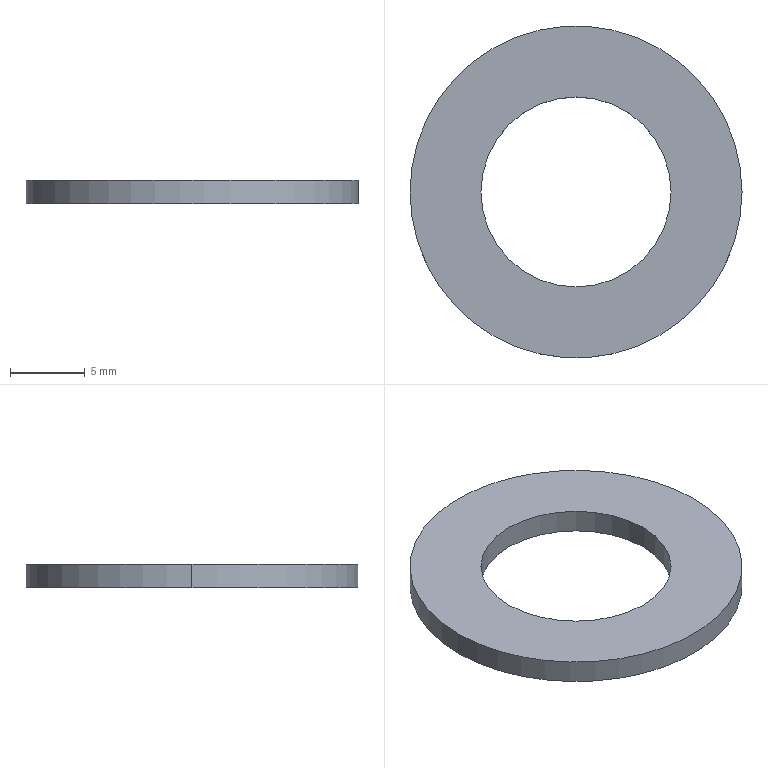Part | SolidWorks | features Extrusion 1 | 1 solid | 6 faces | box 22.276 x 22.276 x 1.6 mm | volume 419.302 mm3 | cylinder 4 | plane 2 | commonest cylinder face diameters 12.751 x2 22.276 x2
STEP:
#1=CARTESIAN_POINT('',(-0.251,0.,0.063));
#2=VERTEX_POINT('',#1);
#3=CARTESIAN_POINT('',(0.251,0.,0.063));
#4=VERTEX_POINT('',#3);
#5=CARTESIAN_POINT('',(0.,0.,0.063));
#6=DIRECTION('',(0.,0.,1.));
#7=DIRECTION('',(1.,0.,0.));
#8=AXIS2_PLACEMENT_3D('',#5,#6,#7);
#9=CIRCLE('',#8,0.251);
#10=EDGE_CURVE('',#2,#4,#9,.T.);
#11=ORIENTED_EDGE('',*,*,#10,.T.);
#12=CARTESIAN_POINT('',(0.251,0.,0.));
#13=VERTEX_POINT('',#12);
#14=CARTESIAN_POINT('',(0.251,0.,0.063));
#15=DIRECTION('',(0.,0.,-1.));
#16=VECTOR('',#15,39.37);
#17=LINE('',#14,#16);
#18=EDGE_CURVE('',#4,#13,#17,.T.);
#19=ORIENTED_EDGE('',*,*,#18,.T.);
#20=CARTESIAN_POINT('',(-0.251,0.,0.));
#21=VERTEX_POINT('',#20);
#22=CARTESIAN_POINT('',(0.,0.,0.));
#23=DIRECTION('',(0.,0.,1.));
#24=DIRECTION('',(1.,0.,0.));
#25=AXIS2_PLACEMENT_3D('',#22,#23,#24);
#26=CIRCLE('',#25,0.251);
#27=EDGE_CURVE('',#21,#13,#26,.T.);
#28=ORIENTED_EDGE('',*,*,#27,.F.);
#29=CARTESIAN_POINT('',(-0.251,0.,0.063));
#30=DIRECTION('',(0.,0.,-1.));
#31=VECTOR('',#30,39.37);
#32=LINE('',#29,#31);
#33=EDGE_CURVE('',#2,#21,#32,.T.);
#34=ORIENTED_EDGE('',*,*,#33,.F.);
#35=EDGE_LOOP('',(#11,#19,#28,#34));
#36=FACE_OUTER_BOUND('',#35,.T.);
#37=CARTESIAN_POINT('',(0.,0.,0.063));
#38=DIRECTION('',(0.,0.,-1.));
#39=DIRECTION('',(-1.,0.,0.));
#40=AXIS2_PLACEMENT_3D('',#37,#38,#39);
#41=CYLINDRICAL_SURFACE('',#40,0.251);
#42=ADVANCED_FACE('',(#36),#41,.F.);
#43=CARTESIAN_POINT('',(0.4385,0.,0.063));
#44=VERTEX_POINT('',#43);
#45=CARTESIAN_POINT('',(-0.4385,0.,0.063));
#46=VERTEX_POINT('',#45);
#47=CARTESIAN_POINT('',(0.,0.,0.063));
#48=DIRECTION('',(0.,0.,1.));
#49=DIRECTION('',(1.,0.,0.));
#50=AXIS2_PLACEMENT_3D('',#47,#48,#49);
#51=CIRCLE('',#50,0.4385);
#52=EDGE_CURVE('',#44,#46,#51,.T.);
#53=ORIENTED_EDGE('',*,*,#52,.F.);
#54=CARTESIAN_POINT('',(0.4385,0.,0.));
#55=VERTEX_POINT('',#54);
#56=CARTESIAN_POINT('',(0.4385,0.,0.063));
#57=DIRECTION('',(0.,0.,-1.));
#58=VECTOR('',#57,39.37);
#59=LINE('',#56,#58);
#60=EDGE_CURVE('',#44,#55,#59,.T.);
#61=ORIENTED_EDGE('',*,*,#60,.T.);
#62=CARTESIAN_POINT('',(-0.4385,0.,0.));
#63=VERTEX_POINT('',#62);
#64=CARTESIAN_POINT('',(0.,0.,0.));
#65=DIRECTION('',(0.,0.,1.));
#66=DIRECTION('',(1.,0.,0.));
#67=AXIS2_PLACEMENT_3D('',#64,#65,#66);
#68=CIRCLE('',#67,0.4385);
#69=EDGE_CURVE('',#55,#63,#68,.T.);
#70=ORIENTED_EDGE('',*,*,#69,.T.);
#71=CARTESIAN_POINT('',(-0.4385,0.,0.063));
#72=DIRECTION('',(0.,0.,-1.));
#73=VECTOR('',#72,39.37);
#74=LINE('',#71,#73);
#75=EDGE_CURVE('',#46,#63,#74,.T.);
#76=ORIENTED_EDGE('',*,*,#75,.F.);
#77=EDGE_LOOP('',(#53,#61,#70,#76));
#78=FACE_OUTER_BOUND('',#77,.T.);
#79=CARTESIAN_POINT('',(0.,0.,0.063));
#80=DIRECTION('',(0.,0.,-1.));
#81=DIRECTION('',(-1.,0.,0.));
#82=AXIS2_PLACEMENT_3D('',#79,#80,#81);
#83=CYLINDRICAL_SURFACE('',#82,0.4385);
#84=ADVANCED_FACE('',(#78),#83,.T.);
#85=CARTESIAN_POINT('',(0.,0.,0.063));
#86=DIRECTION('',(0.,0.,1.));
#87=DIRECTION('',(1.,0.,0.));
#88=AXIS2_PLACEMENT_3D('',#85,#86,#87);
#89=CIRCLE('',#88,0.4385);
#90=EDGE_CURVE('',#46,#44,#89,.T.);
#91=ORIENTED_EDGE('',*,*,#90,.T.);
#92=ORIENTED_EDGE('',*,*,#52,.T.);
#93=EDGE_LOOP('',(#91,#92));
#94=FACE_OUTER_BOUND('',#93,.T.);
#95=ORIENTED_EDGE('',*,*,#10,.F.);
#96=CARTESIAN_POINT('',(0.,0.,0.063));
#97=DIRECTION('',(0.,0.,1.));
#98=DIRECTION('',(1.,0.,0.));
#99=AXIS2_PLACEMENT_3D('',#96,#97,#98);
#100=CIRCLE('',#99,0.251);
#101=EDGE_CURVE('',#4,#2,#100,.T.);
#102=ORIENTED_EDGE('',*,*,#101,.F.);
#103=EDGE_LOOP('',(#95,#102));
#104=FACE_BOUND('',#103,.T.);
#105=CARTESIAN_POINT('',(0.,0.,0.063));
#106=DIRECTION('',(0.,0.,1.));
#107=DIRECTION('',(1.,0.,0.));
#108=AXIS2_PLACEMENT_3D('',#105,#106,#107);
#109=PLANE('',#108);
#110=ADVANCED_FACE('',(#94,#104),#109,.T.);
#111=CARTESIAN_POINT('',(0.,0.,0.));
#112=DIRECTION('',(0.,0.,1.));
#113=DIRECTION('',(1.,0.,0.));
#114=AXIS2_PLACEMENT_3D('',#111,#112,#113);
#115=CIRCLE('',#114,0.4385);
#116=EDGE_CURVE('',#63,#55,#115,.T.);
#117=ORIENTED_EDGE('',*,*,#116,.F.);
#118=ORIENTED_EDGE('',*,*,#69,.F.);
#119=EDGE_LOOP('',(#117,#118));
#120=FACE_OUTER_BOUND('',#119,.T.);
#121=ORIENTED_EDGE('',*,*,#27,.T.);
#122=CARTESIAN_POINT('',(0.,0.,0.));
#123=DIRECTION('',(0.,0.,1.));
#124=DIRECTION('',(1.,0.,0.));
#125=AXIS2_PLACEMENT_3D('',#122,#123,#124);
#126=CIRCLE('',#125,0.251);
#127=EDGE_CURVE('',#13,#21,#126,.T.);
#128=ORIENTED_EDGE('',*,*,#127,.T.);
#129=EDGE_LOOP('',(#121,#128));
#130=FACE_BOUND('',#129,.T.);
#131=CARTESIAN_POINT('',(0.,0.,0.));
#132=DIRECTION('',(0.,0.,1.));
#133=DIRECTION('',(1.,0.,0.));
#134=AXIS2_PLACEMENT_3D('',#131,#132,#133);
#135=PLANE('',#134);
#136=ADVANCED_FACE('',(#120,#130),#135,.F.);
#137=ORIENTED_EDGE('',*,*,#60,.F.);
#138=ORIENTED_EDGE('',*,*,#90,.F.);
#139=ORIENTED_EDGE('',*,*,#75,.T.);
#140=ORIENTED_EDGE('',*,*,#116,.T.);
#141=EDGE_LOOP('',(#137,#138,#139,#140));
#142=FACE_OUTER_BOUND('',#141,.T.);
#143=CARTESIAN_POINT('',(0.,0.,0.063));
#144=DIRECTION('',(0.,0.,-1.));
#145=DIRECTION('',(-1.,0.,0.));
#146=AXIS2_PLACEMENT_3D('',#143,#144,#145);
#147=CYLINDRICAL_SURFACE('',#146,0.4385);
#148=ADVANCED_FACE('',(#142),#147,.T.);
#149=ORIENTED_EDGE('',*,*,#18,.F.);
#150=ORIENTED_EDGE('',*,*,#101,.T.);
#151=ORIENTED_EDGE('',*,*,#33,.T.);
#152=ORIENTED_EDGE('',*,*,#127,.F.);
#153=EDGE_LOOP('',(#149,#150,#151,#152));
#154=FACE_OUTER_BOUND('',#153,.T.);
#155=CARTESIAN_POINT('',(0.,0.,0.063));
#156=DIRECTION('',(0.,0.,-1.));
#157=DIRECTION('',(-1.,0.,0.));
#158=AXIS2_PLACEMENT_3D('',#155,#156,#157);
#159=CYLINDRICAL_SURFACE('',#158,0.251);
#160=ADVANCED_FACE('',(#154),#159,.F.);
#161=CLOSED_SHELL('',(#42,#84,#110,#136,#148,#160));
#162=MANIFOLD_SOLID_BREP('',#161);
#163=CARTESIAN_POINT('',(0.,0.,0.));
#164=DIRECTION('',(0.,0.,1.));
#165=DIRECTION('',(1.,0.,0.));
#166=AXIS2_PLACEMENT_3D('',#163,#164,#165);
#167=(LENGTH_UNIT()NAMED_UNIT(*)SI_UNIT($,.METRE.));
#168=LENGTH_MEASURE_WITH_UNIT(LENGTH_MEASURE(0.0254),#167);
#169=DIMENSIONAL_EXPONENTS(1.,0.,0.,0.,0.,0.,0.);
#170=(CONVERSION_BASED_UNIT('INCH',#168)LENGTH_UNIT()NAMED_UNIT(#169));
#171=UNCERTAINTY_MEASURE_WITH_UNIT(LENGTH_MEASURE(0.00001),#170,'','');
#172=(NAMED_UNIT(*)PLANE_ANGLE_UNIT()SI_UNIT($,.RADIAN.));
#173=(NAMED_UNIT(*)SI_UNIT($,.STERADIAN.)SOLID_ANGLE_UNIT());
#174=(GEOMETRIC_REPRESENTATION_CONTEXT(3)GLOBAL_UNCERTAINTY_ASSIGNED_CONTEXT((#171))GLOBAL_UNIT_ASSIGNED_CONTEXT((#170,#172,#173))REPRESENTATION_CONTEXT('',''));
#175=ADVANCED_BREP_SHAPE_REPRESENTATION('',(#162,#166),#174);